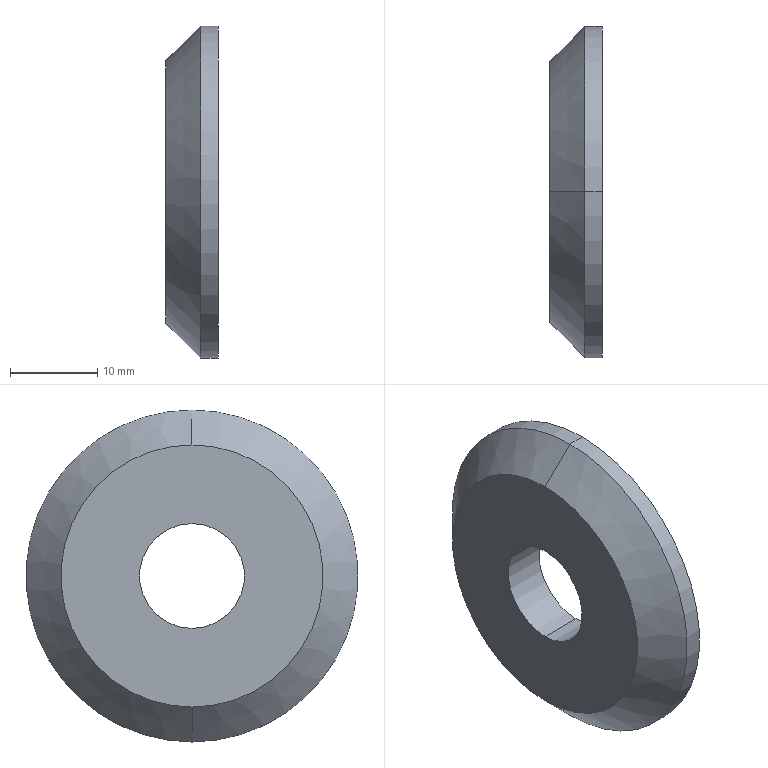Part | SolidWorks | features Revolution 1 | 1 solid | 11 faces | box 6 x 38 x 38 mm | volume 4644 mm3 | cylinder 6 | plane 3 | cone 2 | commonest cylinder face diameters 12 x2 30 x2 38 x2
STEP:
#1=CARTESIAN_POINT('',(3.,0.,19.));
#2=VERTEX_POINT('',#1);
#3=CARTESIAN_POINT('',(3.,0.,-19.));
#4=VERTEX_POINT('',#3);
#5=CARTESIAN_POINT('',(3.,0.,0.));
#6=DIRECTION('',(-1.,0.,0.));
#7=DIRECTION('',(0.,0.,1.));
#8=AXIS2_PLACEMENT_3D('',#5,#6,#7);
#9=CIRCLE('',#8,19.);
#10=EDGE_CURVE('',#2,#4,#9,.T.);
#11=ORIENTED_EDGE('',*,*,#10,.T.);
#12=CARTESIAN_POINT('',(1.,0.,-19.));
#13=VERTEX_POINT('',#12);
#14=CARTESIAN_POINT('',(-11.26,0.,-19.));
#15=DIRECTION('',(-1.,0.,0.));
#16=VECTOR('',#15,1000.);
#17=LINE('',#14,#16);
#18=EDGE_CURVE('',#4,#13,#17,.T.);
#19=ORIENTED_EDGE('',*,*,#18,.T.);
#20=CARTESIAN_POINT('',(1.,0.,19.));
#21=VERTEX_POINT('',#20);
#22=CARTESIAN_POINT('',(1.,0.,0.));
#23=DIRECTION('',(-1.,0.,0.));
#24=DIRECTION('',(0.,0.,1.));
#25=AXIS2_PLACEMENT_3D('',#22,#23,#24);
#26=CIRCLE('',#25,19.);
#27=EDGE_CURVE('',#21,#13,#26,.T.);
#28=ORIENTED_EDGE('',*,*,#27,.F.);
#29=CARTESIAN_POINT('',(-11.26,0.,19.));
#30=DIRECTION('',(-1.,0.,0.));
#31=VECTOR('',#30,1000.);
#32=LINE('',#29,#31);
#33=EDGE_CURVE('',#2,#21,#32,.T.);
#34=ORIENTED_EDGE('',*,*,#33,.F.);
#35=EDGE_LOOP('',(#11,#19,#28,#34));
#36=FACE_OUTER_BOUND('',#35,.T.);
#37=CARTESIAN_POINT('',(-11.26,0.,0.));
#38=DIRECTION('',(-1.,0.,0.));
#39=DIRECTION('',(0.,0.,1.));
#40=AXIS2_PLACEMENT_3D('',#37,#38,#39);
#41=CYLINDRICAL_SURFACE('',#40,19.);
#42=ADVANCED_FACE('',(#36),#41,.T.);
#43=CARTESIAN_POINT('',(-3.,0.,15.));
#44=VERTEX_POINT('',#43);
#45=CARTESIAN_POINT('',(-3.,0.,-15.));
#46=VERTEX_POINT('',#45);
#47=CARTESIAN_POINT('',(-3.,0.,0.));
#48=DIRECTION('',(-1.,0.,0.));
#49=DIRECTION('',(0.,0.,1.));
#50=AXIS2_PLACEMENT_3D('',#47,#48,#49);
#51=CIRCLE('',#50,15.);
#52=EDGE_CURVE('',#44,#46,#51,.T.);
#53=ORIENTED_EDGE('',*,*,#52,.F.);
#54=CARTESIAN_POINT('',(1.,0.,19.));
#55=DIRECTION('',(0.7071,0.,0.7071));
#56=VECTOR('',#55,1000.);
#57=LINE('',#54,#56);
#58=EDGE_CURVE('',#44,#21,#57,.T.);
#59=ORIENTED_EDGE('',*,*,#58,.T.);
#60=ORIENTED_EDGE('',*,*,#27,.T.);
#61=CARTESIAN_POINT('',(1.,0.,-19.));
#62=DIRECTION('',(0.7071,0.,-0.7071));
#63=VECTOR('',#62,1000.);
#64=LINE('',#61,#63);
#65=EDGE_CURVE('',#46,#13,#64,.T.);
#66=ORIENTED_EDGE('',*,*,#65,.F.);
#67=EDGE_LOOP('',(#53,#59,#60,#66));
#68=FACE_OUTER_BOUND('',#67,.T.);
#69=CARTESIAN_POINT('',(1.,0.,0.));
#70=DIRECTION('',(1.,0.,0.));
#71=DIRECTION('',(0.,0.,-1.));
#72=AXIS2_PLACEMENT_3D('',#69,#70,#71);
#73=CONICAL_SURFACE('',#72,19.,0.7854);
#74=ADVANCED_FACE('',(#68),#73,.T.);
#75=CARTESIAN_POINT('',(2.,0.,-6.));
#76=VERTEX_POINT('',#75);
#77=CARTESIAN_POINT('',(2.,0.,6.));
#78=VERTEX_POINT('',#77);
#79=CARTESIAN_POINT('',(2.,0.,0.));
#80=DIRECTION('',(-1.,0.,0.));
#81=DIRECTION('',(0.,0.,1.));
#82=AXIS2_PLACEMENT_3D('',#79,#80,#81);
#83=CIRCLE('',#82,6.);
#84=EDGE_CURVE('',#76,#78,#83,.T.);
#85=ORIENTED_EDGE('',*,*,#84,.F.);
#86=CARTESIAN_POINT('',(-3.,0.,-6.));
#87=VERTEX_POINT('',#86);
#88=CARTESIAN_POINT('',(-11.26,0.,-6.));
#89=DIRECTION('',(-1.,0.,0.));
#90=VECTOR('',#89,1000.);
#91=LINE('',#88,#90);
#92=EDGE_CURVE('',#76,#87,#91,.T.);
#93=ORIENTED_EDGE('',*,*,#92,.T.);
#94=CARTESIAN_POINT('',(-3.,0.,6.));
#95=VERTEX_POINT('',#94);
#96=CARTESIAN_POINT('',(-3.,0.,0.));
#97=DIRECTION('',(-1.,0.,0.));
#98=DIRECTION('',(0.,0.,1.));
#99=AXIS2_PLACEMENT_3D('',#96,#97,#98);
#100=CIRCLE('',#99,6.);
#101=EDGE_CURVE('',#87,#95,#100,.T.);
#102=ORIENTED_EDGE('',*,*,#101,.T.);
#103=CARTESIAN_POINT('',(-11.26,0.,6.));
#104=DIRECTION('',(-1.,0.,0.));
#105=VECTOR('',#104,1000.);
#106=LINE('',#103,#105);
#107=EDGE_CURVE('',#78,#95,#106,.T.);
#108=ORIENTED_EDGE('',*,*,#107,.F.);
#109=EDGE_LOOP('',(#85,#93,#102,#108));
#110=FACE_OUTER_BOUND('',#109,.T.);
#111=CARTESIAN_POINT('',(-11.26,0.,0.));
#112=DIRECTION('',(-1.,0.,0.));
#113=DIRECTION('',(0.,0.,1.));
#114=AXIS2_PLACEMENT_3D('',#111,#112,#113);
#115=CYLINDRICAL_SURFACE('',#114,6.);
#116=ADVANCED_FACE('',(#110),#115,.F.);
#117=CARTESIAN_POINT('',(3.,0.,-15.));
#118=VERTEX_POINT('',#117);
#119=CARTESIAN_POINT('',(3.,0.,15.));
#120=VERTEX_POINT('',#119);
#121=CARTESIAN_POINT('',(3.,0.,0.));
#122=DIRECTION('',(-1.,0.,0.));
#123=DIRECTION('',(0.,0.,1.));
#124=AXIS2_PLACEMENT_3D('',#121,#122,#123);
#125=CIRCLE('',#124,15.);
#126=EDGE_CURVE('',#118,#120,#125,.T.);
#127=ORIENTED_EDGE('',*,*,#126,.F.);
#128=CARTESIAN_POINT('',(2.,0.,-15.));
#129=VERTEX_POINT('',#128);
#130=CARTESIAN_POINT('',(-11.26,0.,-15.));
#131=DIRECTION('',(-1.,0.,0.));
#132=VECTOR('',#131,1000.);
#133=LINE('',#130,#132);
#134=EDGE_CURVE('',#118,#129,#133,.T.);
#135=ORIENTED_EDGE('',*,*,#134,.T.);
#136=CARTESIAN_POINT('',(2.,0.,15.));
#137=VERTEX_POINT('',#136);
#138=CARTESIAN_POINT('',(2.,0.,0.));
#139=DIRECTION('',(-1.,0.,0.));
#140=DIRECTION('',(0.,0.,1.));
#141=AXIS2_PLACEMENT_3D('',#138,#139,#140);
#142=CIRCLE('',#141,15.);
#143=EDGE_CURVE('',#129,#137,#142,.T.);
#144=ORIENTED_EDGE('',*,*,#143,.T.);
#145=CARTESIAN_POINT('',(-11.26,0.,15.));
#146=DIRECTION('',(-1.,0.,0.));
#147=VECTOR('',#146,1000.);
#148=LINE('',#145,#147);
#149=EDGE_CURVE('',#120,#137,#148,.T.);
#150=ORIENTED_EDGE('',*,*,#149,.F.);
#151=EDGE_LOOP('',(#127,#135,#144,#150));
#152=FACE_OUTER_BOUND('',#151,.T.);
#153=CARTESIAN_POINT('',(-11.26,0.,0.));
#154=DIRECTION('',(-1.,0.,0.));
#155=DIRECTION('',(0.,0.,1.));
#156=AXIS2_PLACEMENT_3D('',#153,#154,#155);
#157=CYLINDRICAL_SURFACE('',#156,15.);
#158=ADVANCED_FACE('',(#152),#157,.F.);
#159=ORIENTED_EDGE('',*,*,#134,.F.);
#160=CARTESIAN_POINT('',(3.,0.,0.));
#161=DIRECTION('',(-1.,0.,0.));
#162=DIRECTION('',(0.,0.,1.));
#163=AXIS2_PLACEMENT_3D('',#160,#161,#162);
#164=CIRCLE('',#163,15.);
#165=EDGE_CURVE('',#120,#118,#164,.T.);
#166=ORIENTED_EDGE('',*,*,#165,.F.);
#167=ORIENTED_EDGE('',*,*,#149,.T.);
#168=CARTESIAN_POINT('',(2.,0.,0.));
#169=DIRECTION('',(-1.,0.,0.));
#170=DIRECTION('',(0.,0.,1.));
#171=AXIS2_PLACEMENT_3D('',#168,#169,#170);
#172=CIRCLE('',#171,15.);
#173=EDGE_CURVE('',#137,#129,#172,.T.);
#174=ORIENTED_EDGE('',*,*,#173,.T.);
#175=EDGE_LOOP('',(#159,#166,#167,#174));
#176=FACE_OUTER_BOUND('',#175,.T.);
#177=CARTESIAN_POINT('',(-11.26,0.,0.));
#178=DIRECTION('',(-1.,0.,0.));
#179=DIRECTION('',(0.,0.,1.));
#180=AXIS2_PLACEMENT_3D('',#177,#178,#179);
#181=CYLINDRICAL_SURFACE('',#180,15.);
#182=ADVANCED_FACE('',(#176),#181,.F.);
#183=ORIENTED_EDGE('',*,*,#173,.F.);
#184=ORIENTED_EDGE('',*,*,#143,.F.);
#185=EDGE_LOOP('',(#183,#184));
#186=FACE_OUTER_BOUND('',#185,.T.);
#187=CARTESIAN_POINT('',(2.,0.,0.));
#188=DIRECTION('',(-1.,0.,0.));
#189=DIRECTION('',(0.,0.,1.));
#190=AXIS2_PLACEMENT_3D('',#187,#188,#189);
#191=CIRCLE('',#190,6.);
#192=EDGE_CURVE('',#78,#76,#191,.T.);
#193=ORIENTED_EDGE('',*,*,#192,.T.);
#194=ORIENTED_EDGE('',*,*,#84,.T.);
#195=EDGE_LOOP('',(#193,#194));
#196=FACE_BOUND('',#195,.T.);
#197=CARTESIAN_POINT('',(2.,15.,0.));
#198=DIRECTION('',(-1.,0.,0.));
#199=DIRECTION('',(0.,0.,1.));
#200=AXIS2_PLACEMENT_3D('',#197,#198,#199);
#201=PLANE('',#200);
#202=ADVANCED_FACE('',(#186,#196),#201,.F.);
#203=ORIENTED_EDGE('',*,*,#92,.F.);
#204=ORIENTED_EDGE('',*,*,#192,.F.);
#205=ORIENTED_EDGE('',*,*,#107,.T.);
#206=CARTESIAN_POINT('',(-3.,0.,0.));
#207=DIRECTION('',(-1.,0.,0.));
#208=DIRECTION('',(0.,0.,1.));
#209=AXIS2_PLACEMENT_3D('',#206,#207,#208);
#210=CIRCLE('',#209,6.);
#211=EDGE_CURVE('',#95,#87,#210,.T.);
#212=ORIENTED_EDGE('',*,*,#211,.T.);
#213=EDGE_LOOP('',(#203,#204,#205,#212));
#214=FACE_OUTER_BOUND('',#213,.T.);
#215=CARTESIAN_POINT('',(-11.26,0.,0.));
#216=DIRECTION('',(-1.,0.,0.));
#217=DIRECTION('',(0.,0.,1.));
#218=AXIS2_PLACEMENT_3D('',#215,#216,#217);
#219=CYLINDRICAL_SURFACE('',#218,6.);
#220=ADVANCED_FACE('',(#214),#219,.F.);
#221=ORIENTED_EDGE('',*,*,#211,.F.);
#222=ORIENTED_EDGE('',*,*,#101,.F.);
#223=EDGE_LOOP('',(#221,#222));
#224=FACE_BOUND('',#223,.T.);
#225=CARTESIAN_POINT('',(-3.,0.,0.));
#226=DIRECTION('',(-1.,0.,0.));
#227=DIRECTION('',(0.,0.,1.));
#228=AXIS2_PLACEMENT_3D('',#225,#226,#227);
#229=CIRCLE('',#228,15.);
#230=EDGE_CURVE('',#46,#44,#229,.T.);
#231=ORIENTED_EDGE('',*,*,#230,.T.);
#232=ORIENTED_EDGE('',*,*,#52,.T.);
#233=EDGE_LOOP('',(#231,#232));
#234=FACE_OUTER_BOUND('',#233,.T.);
#235=CARTESIAN_POINT('',(-3.,15.,0.));
#236=DIRECTION('',(1.,0.,0.));
#237=DIRECTION('',(0.,0.,-1.));
#238=AXIS2_PLACEMENT_3D('',#235,#236,#237);
#239=PLANE('',#238);
#240=ADVANCED_FACE('',(#224,#234),#239,.F.);
#241=ORIENTED_EDGE('',*,*,#58,.F.);
#242=ORIENTED_EDGE('',*,*,#230,.F.);
#243=ORIENTED_EDGE('',*,*,#65,.T.);
#244=CARTESIAN_POINT('',(1.,0.,0.));
#245=DIRECTION('',(-1.,0.,0.));
#246=DIRECTION('',(0.,0.,1.));
#247=AXIS2_PLACEMENT_3D('',#244,#245,#246);
#248=CIRCLE('',#247,19.);
#249=EDGE_CURVE('',#13,#21,#248,.T.);
#250=ORIENTED_EDGE('',*,*,#249,.T.);
#251=EDGE_LOOP('',(#241,#242,#243,#250));
#252=FACE_OUTER_BOUND('',#251,.T.);
#253=CARTESIAN_POINT('',(1.,0.,0.));
#254=DIRECTION('',(1.,0.,0.));
#255=DIRECTION('',(0.,0.,-1.));
#256=AXIS2_PLACEMENT_3D('',#253,#254,#255);
#257=CONICAL_SURFACE('',#256,19.,0.7854);
#258=ADVANCED_FACE('',(#252),#257,.T.);
#259=ORIENTED_EDGE('',*,*,#18,.F.);
#260=CARTESIAN_POINT('',(3.,0.,0.));
#261=DIRECTION('',(-1.,0.,0.));
#262=DIRECTION('',(0.,0.,1.));
#263=AXIS2_PLACEMENT_3D('',#260,#261,#262);
#264=CIRCLE('',#263,19.);
#265=EDGE_CURVE('',#4,#2,#264,.T.);
#266=ORIENTED_EDGE('',*,*,#265,.T.);
#267=ORIENTED_EDGE('',*,*,#33,.T.);
#268=ORIENTED_EDGE('',*,*,#249,.F.);
#269=EDGE_LOOP('',(#259,#266,#267,#268));
#270=FACE_OUTER_BOUND('',#269,.T.);
#271=CARTESIAN_POINT('',(-11.26,0.,0.));
#272=DIRECTION('',(-1.,0.,0.));
#273=DIRECTION('',(0.,0.,1.));
#274=AXIS2_PLACEMENT_3D('',#271,#272,#273);
#275=CYLINDRICAL_SURFACE('',#274,19.);
#276=ADVANCED_FACE('',(#270),#275,.T.);
#277=ORIENTED_EDGE('',*,*,#10,.F.);
#278=ORIENTED_EDGE('',*,*,#265,.F.);
#279=EDGE_LOOP('',(#277,#278));
#280=FACE_OUTER_BOUND('',#279,.T.);
#281=ORIENTED_EDGE('',*,*,#165,.T.);
#282=ORIENTED_EDGE('',*,*,#126,.T.);
#283=EDGE_LOOP('',(#281,#282));
#284=FACE_BOUND('',#283,.T.);
#285=CARTESIAN_POINT('',(3.,19.,0.));
#286=DIRECTION('',(-1.,0.,0.));
#287=DIRECTION('',(0.,0.,1.));
#288=AXIS2_PLACEMENT_3D('',#285,#286,#287);
#289=PLANE('',#288);
#290=ADVANCED_FACE('',(#280,#284),#289,.F.);
#291=CLOSED_SHELL('',(#42,#74,#116,#158,#182,#202,#220,#240,#258,#276,#290));
#292=MANIFOLD_SOLID_BREP('',#291);
#293=CARTESIAN_POINT('',(0.,0.,0.));
#294=DIRECTION('',(0.,0.,1.));
#295=DIRECTION('',(1.,0.,0.));
#296=AXIS2_PLACEMENT_3D('',#293,#294,#295);
#297=(LENGTH_UNIT()NAMED_UNIT(*)SI_UNIT(.MILLI.,.METRE.));
#298=UNCERTAINTY_MEASURE_WITH_UNIT(LENGTH_MEASURE(0.00001),#297,'','');
#299=(NAMED_UNIT(*)PLANE_ANGLE_UNIT()SI_UNIT($,.RADIAN.));
#300=(NAMED_UNIT(*)SI_UNIT($,.STERADIAN.)SOLID_ANGLE_UNIT());
#301=(GEOMETRIC_REPRESENTATION_CONTEXT(3)GLOBAL_UNCERTAINTY_ASSIGNED_CONTEXT((#298))GLOBAL_UNIT_ASSIGNED_CONTEXT((#297,#299,#300))REPRESENTATION_CONTEXT('',''));
#302=ADVANCED_BREP_SHAPE_REPRESENTATION('',(#292,#296),#301);